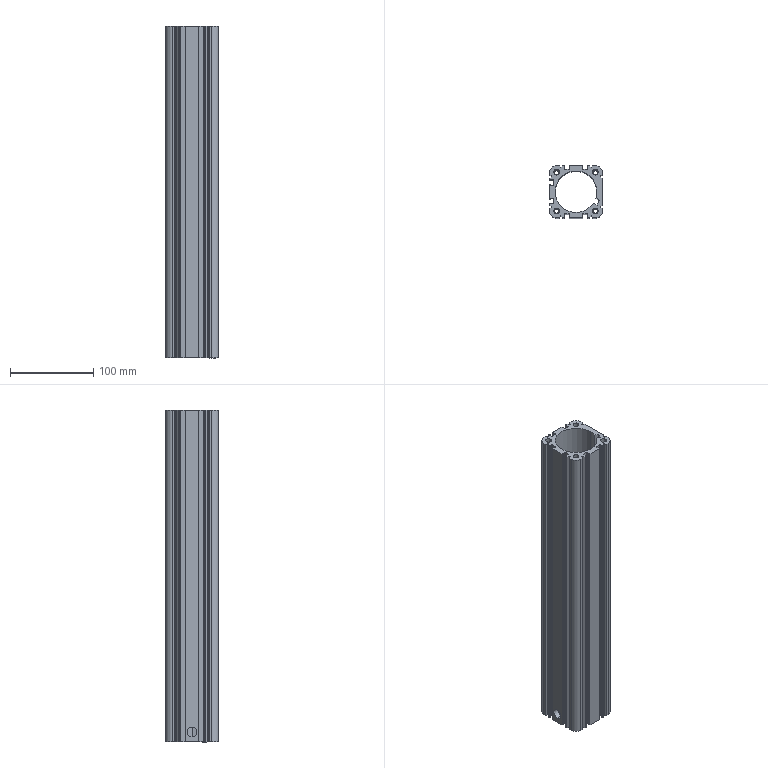Part | SolidWorks | features BaseBody 1 | 1 solid | 204 faces | box 63 x 63 x 398 mm | volume 629539 mm3 | cylinder 107 | plane 81 | cone 16 | commonest cylinder face diameters 1 x38 0.4 x24 6.8 x16 0.8 x12 5.3 x8 16.5 x4